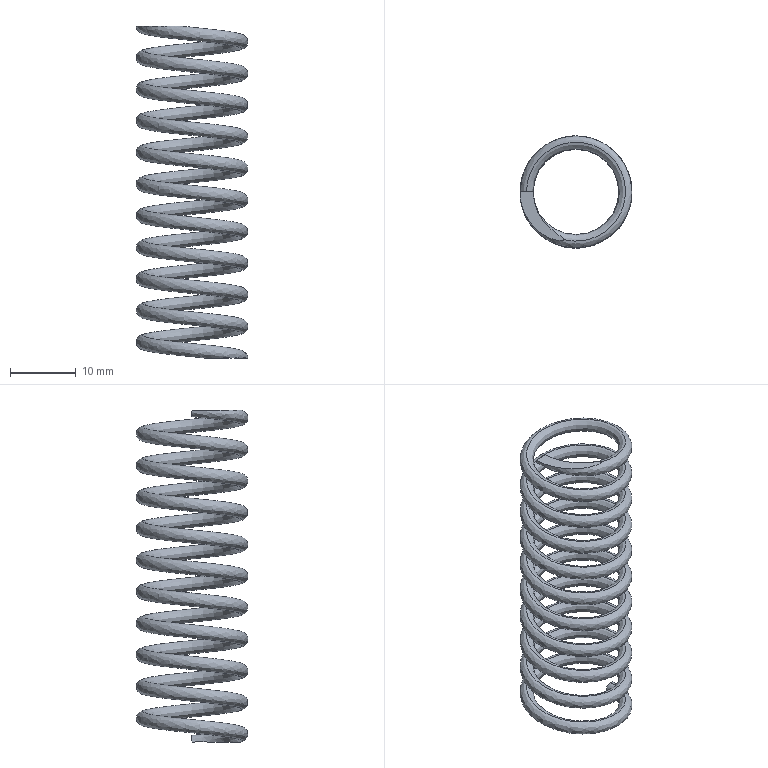Part | STEP file | HB362-65 end not tightened, ground flat 0.25 turns 15×50 | 1 solid | 6 faces | box 17 x 17 x 50.4 mm | volume 1550 mm3 | plane 4 | spline 2